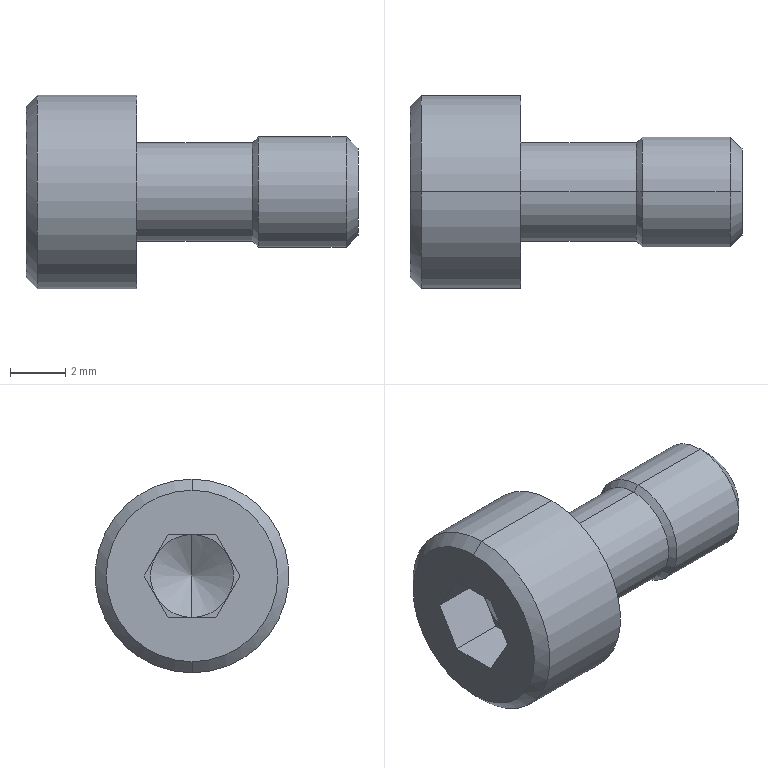Part | STEP file | 0243_Z_SCBS4-8_1 | 1 solid | 29 faces | box 12 x 7 x 7 mm | volume 223.092 mm3 | plane 15 | cone 8 | cylinder 6 | commonest cylinder face diameters 3.57 x2 4 x2 7 x2